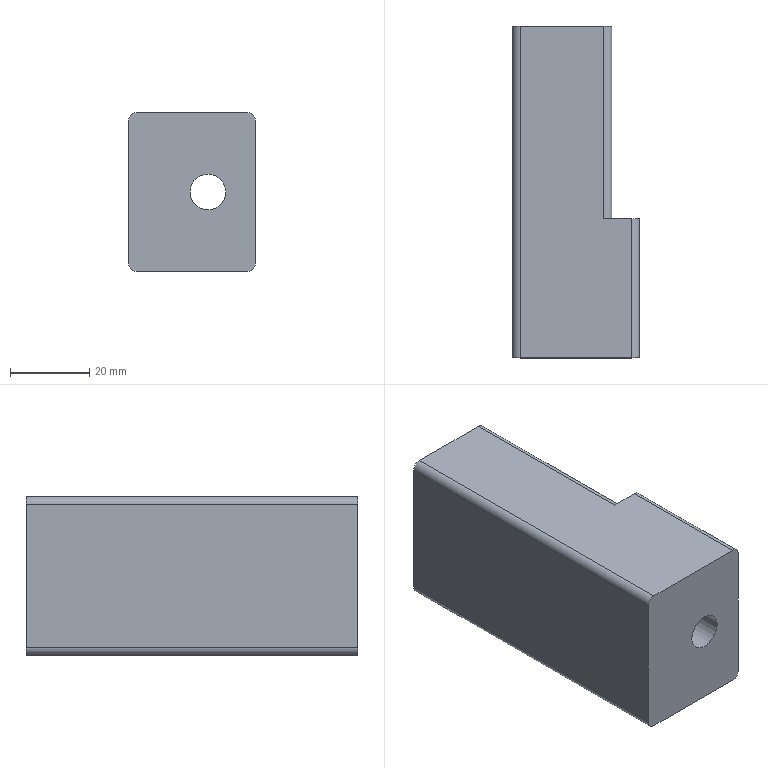NC program | Mastercam | posted with a generic post | part box 32 x 83.5 x 40 mm
Lines 1603 to 2565 of 4494:
(10 FEM |TOOL - 9|DIA. OFF. - 9|LEN. - 9|TOOL DIA. - 10.)
N3262 T9 M6
N3264 G0 G54 G90 X.244 Y-22.653 C0. B0. S7000 M3
N3266 G43 H9 Z50.
N3268 Z1.
N3270 G1 Z-.499 F600.
N3272 X4.744 Y-5.225 F3000.
N3274 G3 X4.9 Y-4. I-4.744 J1.225
N3276 X0. Y.9 I-4.9
N3278 X-4.9 Y-4. J-4.9
N3280 X-4.744 Y-5.225 I4.9
N3282 G1 X-.244 Y-22.653
N3284 Z-.998 F600.
N3286 X-4.744 Y-5.225 F3000.
N3288 G2 X-4.9 Y-4. I4.744 J1.225
N3290 X0. Y.9 I4.9
N3292 X4.9 Y-4. J-4.9
N3294 X4.744 Y-5.225 I-4.9
N3296 G1 X.244 Y-22.653
N3298 Z-1.497 F600.
N3300 X4.744 Y-5.225 F3000.
N3302 G3 X4.9 Y-4. I-4.744 J1.225
N3304 X0. Y.9 I-4.9
N3306 X-4.9 Y-4. J-4.9
N3308 X-4.744 Y-5.225 I4.9
N3310 G1 X-.244 Y-22.653
N3312 Z-1.996 F600.
N3314 X-4.744 Y-5.225 F3000.
N3316 G2 X-4.9 Y-4. I4.744 J1.225
N3318 X0. Y.9 I4.9
N3320 X4.9 Y-4. J-4.9
N3322 X4.744 Y-5.225 I-4.9
N3324 G1 X.244 Y-22.653
N3326 Z-2.495 F600.
N3328 X4.744 Y-5.225 F3000.
N3330 G3 X4.9 Y-4. I-4.744 J1.225
N3332 X0. Y.9 I-4.9
N3334 X-4.9 Y-4. J-4.9
N3336 X-4.744 Y-5.225 I4.9
N3338 G1 X-.244 Y-22.653
N3340 Z-2.994 F600.
N3342 X-4.744 Y-5.225 F3000.
N3344 G2 X-4.9 Y-4. I4.744 J1.225
N3346 X0. Y.9 I4.9
N3348 X4.9 Y-4. J-4.9
N3350 X4.744 Y-5.225 I-4.9
N3352 G1 X.244 Y-22.653
N3354 Z-3.493 F600.
N3356 X4.744 Y-5.225 F3000.
N3358 G3 X4.9 Y-4. I-4.744 J1.225
N3360 X0. Y.9 I-4.9
N3362 X-4.9 Y-4. J-4.9
N3364 X-4.744 Y-5.225 I4.9
N3366 G1 X-.244 Y-22.653
N3368 Z-3.992 F600.
N3370 X-4.744 Y-5.225 F3000.
N3372 G2 X-4.9 Y-4. I4.744 J1.225
N3374 X0. Y.9 I4.9
N3376 X4.9 Y-4. J-4.9
N3378 X4.744 Y-5.225 I-4.9
N3380 G1 X.244 Y-22.653
N3382 Z-4.491 F600.
N3384 X4.744 Y-5.225 F3000.
N3386 G3 X4.9 Y-4. I-4.744 J1.225
N3388 X0. Y.9 I-4.9
N3390 X-4.9 Y-4. J-4.9
N3392 X-4.744 Y-5.225 I4.9
N3394 G1 X-.244 Y-22.653
N3396 Z-4.99 F600.
N3398 X-4.744 Y-5.225 F3000.
N3400 G2 X-4.9 Y-4. I4.744 J1.225
N3402 X0. Y.9 I4.9
N3404 X4.9 Y-4. J-4.9
N3406 X4.744 Y-5.225 I-4.9
N3408 G1 X.244 Y-22.653
N3410 Z-5.489 F600.
N3412 X4.744 Y-5.225 F3000.
N3414 G3 X4.9 Y-4. I-4.744 J1.225
N3416 X0. Y.9 I-4.9
N3418 X-4.9 Y-4. J-4.9
N3420 X-4.744 Y-5.225 I4.9
N3422 G1 X-.244 Y-22.653
N3424 Z-5.988 F600.
N3426 X-4.744 Y-5.225 F3000.
N3428 G2 X-4.9 Y-4. I4.744 J1.225
N3430 X0. Y.9 I4.9
N3432 X4.9 Y-4. J-4.9
N3434 X4.744 Y-5.225 I-4.9
N3436 G1 X.244 Y-22.653
N3438 Z-6.487 F600.
N3440 X4.744 Y-5.225 F3000.
N3442 G3 X4.9 Y-4. I-4.744 J1.225
N3444 X0. Y.9 I-4.9
N3446 X-4.9 Y-4. J-4.9
N3448 X-4.744 Y-5.225 I4.9
N3450 G1 X-.244 Y-22.653
N3452 Z-6.986 F600.
N3454 X-4.744 Y-5.225 F3000.
N3456 G2 X-4.9 Y-4. I4.744 J1.225
N3458 X0. Y.9 I4.9
N3460 X4.9 Y-4. J-4.9
N3462 X4.744 Y-5.225 I-4.9
N3464 G1 X.244 Y-22.653
N3466 Z-7.485 F600.
N3468 X4.744 Y-5.225 F3000.
N3470 G3 X4.9 Y-4. I-4.744 J1.225
N3472 X0. Y.9 I-4.9
N3474 X-4.9 Y-4. J-4.9
N3476 X-4.744 Y-5.225 I4.9
N3478 G1 X-.244 Y-22.653
N3480 Z-7.984 F600.
N3482 X-4.744 Y-5.225 F3000.
N3484 G2 X-4.9 Y-4. I4.744 J1.225
N3486 X0. Y.9 I4.9
N3488 X4.9 Y-4. J-4.9
N3490 X4.744 Y-5.225 I-4.9
N3492 G1 X.244 Y-22.653
N3494 Z-8.482 F600.
N3496 X4.744 Y-5.225 F3000.
N3498 G3 X4.9 Y-4. I-4.744 J1.225
N3500 X0. Y.9 I-4.9
N3502 X-4.9 Y-4. J-4.9
N3504 X-4.744 Y-5.225 I4.9
N3506 G1 X-.244 Y-22.653
N3508 Z-8.981 F600.
N3510 X-4.744 Y-5.225 F3000.
N3512 G2 X-4.9 Y-4. I4.744 J1.225
N3514 X0. Y.9 I4.9
N3516 X4.9 Y-4. J-4.9
N3518 X4.744 Y-5.225 I-4.9
N3520 G1 X.244 Y-22.653
N3522 Z-9.48 F600.
N3524 X4.744 Y-5.225 F3000.
N3526 G3 X4.9 Y-4. I-4.744 J1.225
N3528 X0. Y.9 I-4.9
N3530 X-4.9 Y-4. J-4.9
N3532 X-4.744 Y-5.225 I4.9
N3534 G1 X-.244 Y-22.653
N3536 Z-9.979 F600.
N3538 X-4.744 Y-5.225 F3000.
N3540 G2 X-4.9 Y-4. I4.744 J1.225
N3542 X0. Y.9 I4.9
N3544 X4.9 Y-4. J-4.9
N3546 X4.744 Y-5.225 I-4.9
N3548 G1 X.244 Y-22.653
N3550 Z-10.478 F600.
N3552 X4.744 Y-5.225 F3000.
N3554 G3 X4.9 Y-4. I-4.744 J1.225
N3556 X0. Y.9 I-4.9
N3558 X-4.9 Y-4. J-4.9
N3560 X-4.744 Y-5.225 I4.9
N3562 G1 X-.244 Y-22.653
N3564 Z-10.977 F600.
N3566 X-4.744 Y-5.225 F3000.
N3568 G2 X-4.9 Y-4. I4.744 J1.225
N3570 X0. Y.9 I4.9
N3572 X4.9 Y-4. J-4.9
N3574 X4.744 Y-5.225 I-4.9
N3576 G1 X.244 Y-22.653
N3578 Z-11.476 F600.
N3580 X4.744 Y-5.225 F3000.
N3582 G3 X4.9 Y-4. I-4.744 J1.225
N3584 X0. Y.9 I-4.9
N3586 X-4.9 Y-4. J-4.9
N3588 X-4.744 Y-5.225 I4.9
N3590 G1 X-.244 Y-22.653
N3592 Z-11.975 F600.
N3594 X-4.744 Y-5.225 F3000.
N3596 G2 X-4.9 Y-4. I4.744 J1.225
N3598 X0. Y.9 I4.9
N3600 X4.9 Y-4. J-4.9
N3602 X4.744 Y-5.225 I-4.9
N3604 G1 X.244 Y-22.653
N3606 Z-12.474 F600.
N3608 X4.744 Y-5.225 F3000.
N3610 G3 X4.9 Y-4. I-4.744 J1.225
N3612 X0. Y.9 I-4.9
N3614 X-4.9 Y-4. J-4.9
N3616 X-4.744 Y-5.225 I4.9
N3618 G1 X-.244 Y-22.653
N3620 Z-12.973 F600.
N3622 X-4.744 Y-5.225 F3000.
N3624 G2 X-4.9 Y-4. I4.744 J1.225
N3626 X0. Y.9 I4.9
N3628 X4.9 Y-4. J-4.9
N3630 X4.744 Y-5.225 I-4.9
N3632 G1 X.244 Y-22.653
N3634 Z-13.472 F600.
N3636 X4.744 Y-5.225 F3000.
N3638 G3 X4.9 Y-4. I-4.744 J1.225
N3640 X0. Y.9 I-4.9
N3642 X-4.9 Y-4. J-4.9
N3644 X-4.744 Y-5.225 I4.9
N3646 G1 X-.244 Y-22.653
N3648 Z-13.971 F600.
N3650 X-4.744 Y-5.225 F3000.
N3652 G2 X-4.9 Y-4. I4.744 J1.225
N3654 X0. Y.9 I4.9
N3656 X4.9 Y-4. J-4.9
N3658 X4.744 Y-5.225 I-4.9
N3660 G1 X.244 Y-22.653
N3662 Z-14.47 F600.
N3664 X4.744 Y-5.225 F3000.
N3666 G3 X4.9 Y-4. I-4.744 J1.225
N3668 X0. Y.9 I-4.9
N3670 X-4.9 Y-4. J-4.9
N3672 X-4.744 Y-5.225 I4.9
N3674 G1 X-.244 Y-22.653
N3676 Z-14.969 F600.
N3678 X-4.744 Y-5.225 F3000.
N3680 G2 X-4.9 Y-4. I4.744 J1.225
N3682 X0. Y.9 I4.9
N3684 X4.9 Y-4. J-4.9
N3686 X4.744 Y-5.225 I-4.9
N3688 G1 X.244 Y-22.653
N3690 Z-15.468 F600.
N3692 X4.744 Y-5.225 F3000.
N3694 G3 X4.9 Y-4. I-4.744 J1.225
N3696 X0. Y.9 I-4.9
N3698 X-4.9 Y-4. J-4.9
N3700 X-4.744 Y-5.225 I4.9
N3702 G1 X-.244 Y-22.653
N3704 Z-15.967 F600.
N3706 X-4.744 Y-5.225 F3000.
N3708 G2 X-4.9 Y-4. I4.744 J1.225
N3710 X0. Y.9 I4.9
N3712 X4.9 Y-4. J-4.9
N3714 X4.744 Y-5.225 I-4.9
N3716 G1 X.244 Y-22.653
N3718 Z-16.466 F600.
N3720 X4.744 Y-5.225 F3000.
N3722 G3 X4.9 Y-4. I-4.744 J1.225
N3724 X0. Y.9 I-4.9
N3726 X-4.9 Y-4. J-4.9
N3728 X-4.744 Y-5.225 I4.9
N3730 G1 X-.244 Y-22.653
N3732 Z-16.965 F600.
N3734 X-4.744 Y-5.225 F3000.
N3736 G2 X-4.9 Y-4. I4.744 J1.225
N3738 X0. Y.9 I4.9
N3740 X4.9 Y-4. J-4.9
N3742 X4.744 Y-5.225 I-4.9
N3744 G1 X.244 Y-22.653
N3746 Z-17.464 F600.
N3748 X4.744 Y-5.225 F3000.
N3750 G3 X4.9 Y-4. I-4.744 J1.225
N3752 X0. Y.9 I-4.9
N3754 X-4.9 Y-4. J-4.9
N3756 X-4.744 Y-5.225 I4.9
N3758 G1 X-.244 Y-22.653
N3760 Z-17.963 F600.
N3762 X-4.744 Y-5.225 F3000.
N3764 G2 X-4.9 Y-4. I4.744 J1.225
N3766 X0. Y.9 I4.9
N3768 X4.9 Y-4. J-4.9
N3770 X4.744 Y-5.225 I-4.9
N3772 G1 X.244 Y-22.653
N3774 Z-18.462 F600.
N3776 X4.744 Y-5.225 F3000.
N3778 G3 X4.9 Y-4. I-4.744 J1.225
N3780 X0. Y.9 I-4.9
N3782 X-4.9 Y-4. J-4.9
N3784 X-4.744 Y-5.225 I4.9
N3786 G1 X-.244 Y-22.653
N3788 Z-18.961 F600.
N3790 X-4.744 Y-5.225 F3000.
N3792 G2 X-4.9 Y-4. I4.744 J1.225
N3794 X0. Y.9 I4.9
N3796 X4.9 Y-4. J-4.9
N3798 X4.744 Y-5.225 I-4.9
N3800 G1 X.244 Y-22.653
N3802 Z-19.46 F600.
N3804 X4.744 Y-5.225 F3000.
N3806 G3 X4.9 Y-4. I-4.744 J1.225
N3808 X0. Y.9 I-4.9
N3810 X-4.9 Y-4. J-4.9
N3812 X-4.744 Y-5.225 I4.9
N3814 G1 X-.244 Y-22.653
N3816 Z-19.959 F600.
N3818 X-4.744 Y-5.225 F3000.
N3820 G2 X-4.9 Y-4. I4.744 J1.225
N3822 X0. Y.9 I4.9
N3824 X4.9 Y-4. J-4.9
N3826 X4.744 Y-5.225 I-4.9
N3828 G1 X.244 Y-22.653
N3830 Z-20.458 F600.
N3832 X4.744 Y-5.225 F3000.
N3834 G3 X4.9 Y-4. I-4.744 J1.225
N3836 X0. Y.9 I-4.9
N3838 X-4.9 Y-4. J-4.9
N3840 X-4.744 Y-5.225 I4.9
N3842 G1 X-.244 Y-22.653
N3844 Z-20.957 F600.
N3846 X-4.744 Y-5.225 F3000.
N3848 G2 X-4.9 Y-4. I4.744 J1.225
N3850 X0. Y.9 I4.9
N3852 X4.9 Y-4. J-4.9
N3854 X4.744 Y-5.225 I-4.9
N3856 G1 X.244 Y-22.653
N3858 Z-21.456 F600.
N3860 X4.744 Y-5.225 F3000.
N3862 G3 X4.9 Y-4. I-4.744 J1.225
N3864 X0. Y.9 I-4.9
N3866 X-4.9 Y-4. J-4.9
N3868 X-4.744 Y-5.225 I4.9
N3870 G1 X-.244 Y-22.653
N3872 Z-21.955 F600.
N3874 X-4.744 Y-5.225 F3000.
N3876 G2 X-4.9 Y-4. I4.744 J1.225
N3878 X0. Y.9 I4.9
N3880 X4.9 Y-4. J-4.9
N3882 X4.744 Y-5.225 I-4.9
N3884 G1 X.244 Y-22.653
N3886 Z-22.454 F600.
N3888 X4.744 Y-5.225 F3000.
N3890 G3 X4.9 Y-4. I-4.744 J1.225
N3892 X0. Y.9 I-4.9
N3894 X-4.9 Y-4. J-4.9
N3896 X-4.744 Y-5.225 I4.9
N3898 G1 X-.244 Y-22.653
N3900 Z-22.953 F600.
N3902 X-4.744 Y-5.225 F3000.
N3904 G2 X-4.9 Y-4. I4.744 J1.225
N3906 X0. Y.9 I4.9
N3908 X4.9 Y-4. J-4.9
N3910 X4.744 Y-5.225 I-4.9
N3912 G1 X.244 Y-22.653
N3914 Z-23.452 F600.
N3916 X4.744 Y-5.225 F3000.
N3918 G3 X4.9 Y-4. I-4.744 J1.225
N3920 X0. Y.9 I-4.9
N3922 X-4.9 Y-4. J-4.9
N3924 X-4.744 Y-5.225 I4.9
N3926 G1 X-.244 Y-22.653
N3928 Z-23.951 F600.
N3930 X-4.744 Y-5.225 F3000.
N3932 G2 X-4.9 Y-4. I4.744 J1.225
N3934 X0. Y.9 I4.9
N3936 X4.9 Y-4. J-4.9
N3938 X4.744 Y-5.225 I-4.9
N3940 G1 X.244 Y-22.653
N3942 Z-24.449 F600.
N3944 X4.744 Y-5.225 F3000.
N3946 G3 X4.9 Y-4. I-4.744 J1.225
N3948 X0. Y.9 I-4.9
N3950 X-4.9 Y-4. J-4.9
N3952 X-4.744 Y-5.225 I4.9
N3954 G1 X-.244 Y-22.653
N3956 Z-24.948 F600.
N3958 X-4.744 Y-5.225 F3000.
N3960 G2 X-4.9 Y-4. I4.744 J1.225
N3962 X0. Y.9 I4.9
N3964 X4.9 Y-4. J-4.9
N3966 X4.744 Y-5.225 I-4.9
N3968 G1 X.244 Y-22.653
N3970 Z-25.447 F600.
N3972 X4.744 Y-5.225 F3000.
N3974 G3 X4.9 Y-4. I-4.744 J1.225
N3976 X0. Y.9 I-4.9
N3978 X-4.9 Y-4. J-4.9
N3980 X-4.744 Y-5.225 I4.9
N3982 G1 X-.244 Y-22.653
N3984 Z-25.946 F600.
N3986 X-4.744 Y-5.225 F3000.
N3988 G2 X-4.9 Y-4. I4.744 J1.225
N3990 X0. Y.9 I4.9
N3992 X4.9 Y-4. J-4.9
N3994 X4.744 Y-5.225 I-4.9
N3996 G1 X.244 Y-22.653
N3998 Z-26.445 F600.
N4000 X4.744 Y-5.225 F3000.
N4002 G3 X4.9 Y-4. I-4.744 J1.225
N4004 X0. Y.9 I-4.9
N4006 X-4.9 Y-4. J-4.9
N4008 X-4.744 Y-5.225 I4.9
N4010 G1 X-.244 Y-22.653
N4012 Z-26.944 F600.
N4014 X-4.744 Y-5.225 F3000.
N4016 G2 X-4.9 Y-4. I4.744 J1.225
N4018 X0. Y.9 I4.9
N4020 X4.9 Y-4. J-4.9
N4022 X4.744 Y-5.225 I-4.9
N4024 G1 X.244 Y-22.653
N4026 Z-27.443 F600.
N4028 X4.744 Y-5.225 F3000.
N4030 G3 X4.9 Y-4. I-4.744 J1.225
N4032 X0. Y.9 I-4.9
N4034 X-4.9 Y-4. J-4.9
N4036 X-4.744 Y-5.225 I4.9
N4038 G1 X-.244 Y-22.653
N4040 Z-27.942 F600.
N4042 X-4.744 Y-5.225 F3000.
N4044 G2 X-4.9 Y-4. I4.744 J1.225
N4046 X0. Y.9 I4.9
N4048 X4.9 Y-4. J-4.9
N4050 X4.744 Y-5.225 I-4.9
N4052 G1 X.244 Y-22.653
N4054 Z-28.441 F600.
N4056 X4.744 Y-5.225 F3000.
N4058 G3 X4.9 Y-4. I-4.744 J1.225
N4060 X0. Y.9 I-4.9
N4062 X-4.9 Y-4. J-4.9
N4064 X-4.744 Y-5.225 I4.9
N4066 G1 X-.244 Y-22.653
N4068 Z-28.94 F600.
N4070 X-4.744 Y-5.225 F3000.
N4072 G2 X-4.9 Y-4. I4.744 J1.225
N4074 X0. Y.9 I4.9
N4076 X4.9 Y-4. J-4.9
N4078 X4.744 Y-5.225 I-4.9
N4080 G1 X.244 Y-22.653
N4082 Z-29.439 F600.
N4084 X4.744 Y-5.225 F3000.
N4086 G3 X4.9 Y-4. I-4.744 J1.225
N4088 X0. Y.9 I-4.9
N4090 X-4.9 Y-4. J-4.9
N4092 X-4.744 Y-5.225 I4.9
N4094 G1 X-.244 Y-22.653
N4096 Z-29.938 F600.
N4098 X-4.744 Y-5.225 F3000.
N4100 G2 X-4.9 Y-4. I4.744 J1.225
N4102 X0. Y.9 I4.9
N4104 X4.9 Y-4. J-4.9
N4106 X4.744 Y-5.225 I-4.9
N4108 G1 X.244 Y-22.653
N4110 Z-30.437 F600.
N4112 X4.744 Y-5.225 F3000.
N4114 G3 X4.9 Y-4. I-4.744 J1.225
N4116 X0. Y.9 I-4.9
N4118 X-4.9 Y-4. J-4.9
N4120 X-4.744 Y-5.225 I4.9
N4122 G1 X-.244 Y-22.653
N4124 Z-30.936 F600.
N4126 X-4.744 Y-5.225 F3000.
N4128 G2 X-4.9 Y-4. I4.744 J1.225
N4130 X0. Y.9 I4.9
N4132 X4.9 Y-4. J-4.9
N4134 X4.744 Y-5.225 I-4.9
N4136 G1 X.244 Y-22.653
N4138 Z-31.435 F600.
N4140 X4.744 Y-5.225 F3000.
N4142 G3 X4.9 Y-4. I-4.744 J1.225
N4144 X0. Y.9 I-4.9
N4146 X-4.9 Y-4. J-4.9
N4148 X-4.744 Y-5.225 I4.9
N4150 G1 X-.244 Y-22.653
N4152 Z-31.934 F600.
N4154 X-4.744 Y-5.225 F3000.
N4156 G2 X-4.9 Y-4. I4.744 J1.225
N4158 X0. Y.9 I4.9
N4160 X4.9 Y-4. J-4.9
N4162 X4.744 Y-5.225 I-4.9
N4164 G1 X.244 Y-22.653
N4166 Z-32.433 F600.
N4168 X4.744 Y-5.225 F3000.
N4170 G3 X4.9 Y-4. I-4.744 J1.225
N4172 X0. Y.9 I-4.9
N4174 X-4.9 Y-4. J-4.9
N4176 X-4.744 Y-5.225 I4.9
N4178 G1 X-.244 Y-22.653
N4180 Z-32.932 F600.
N4182 X-4.744 Y-5.225 F3000.
N4184 G2 X-4.9 Y-4. I4.744 J1.225
N4186 X0. Y.9 I4.9
N4188 X4.9 Y-4. J-4.9
N4190 X4.744 Y-5.225 I-4.9
N4192 G1 X.244 Y-22.653
N4194 Z-33.431 F600.
N4196 X4.744 Y-5.225 F3000.
N4198 G3 X4.9 Y-4. I-4.744 J1.225
N4200 X0. Y.9 I-4.9
N4202 X-4.9 Y-4. J-4.9
N4204 X-4.744 Y-5.225 I4.9
N4206 G1 X-.244 Y-22.653
N4208 Z-33.93 F600.
N4210 X-4.744 Y-5.225 F3000.
N4212 G2 X-4.9 Y-4. I4.744 J1.225
N4214 X0. Y.9 I4.9
N4216 X4.9 Y-4. J-4.9
N4218 X4.744 Y-5.225 I-4.9
N4220 G1 X.244 Y-22.653
N4222 Z-34.429 F600.
N4224 X4.744 Y-5.225 F3000.
N4226 G3 X4.9 Y-4. I-4.744 J1.225
N4228 X0. Y.9 I-4.9
N4230 X-4.9 Y-4. J-4.9
N4232 X-4.744 Y-5.225 I4.9
N4234 G1 X-.244 Y-22.653
N4236 Z-34.928 F600.
N4238 X-4.744 Y-5.225 F3000.
N4240 G2 X-4.9 Y-4. I4.744 J1.225
N4242 X0. Y.9 I4.9
N4244 X4.9 Y-4. J-4.9
N4246 X4.744 Y-5.225 I-4.9
N4248 G1 X.244 Y-22.653
N4250 Z-35.427 F600.
N4252 X4.744 Y-5.225 F3000.
N4254 G3 X4.9 Y-4. I-4.744 J1.225
N4256 X0. Y.9 I-4.9
N4258 X-4.9 Y-4. J-4.9
N4260 X-4.744 Y-5.225 I4.9
N4262 G1 X-.244 Y-22.653
N4264 Z-35.926 F600.
N4266 X-4.744 Y-5.225 F3000.
N4268 G2 X-4.9 Y-4. I4.744 J1.225
N4270 X0. Y.9 I4.9
N4272 X4.9 Y-4. J-4.9
N4274 X4.744 Y-5.225 I-4.9
N4276 G1 X.244 Y-22.653
N4278 Z-36.425 F600.
N4280 X4.744 Y-5.225 F3000.
N4282 G3 X4.9 Y-4. I-4.744 J1.225
N4284 X0. Y.9 I-4.9
N4286 X-4.9 Y-4. J-4.9
N4288 X-4.744 Y-5.225 I4.9
N4290 G1 X-.244 Y-22.653
N4292 Z-36.924 F600.
N4294 X-4.744 Y-5.225 F3000.
N4296 G2 X-4.9 Y-4. I4.744 J1.225
N4298 X0. Y.9 I4.9
N4300 X4.9 Y-4. J-4.9
N4302 X4.744 Y-5.225 I-4.9
N4304 G1 X.244 Y-22.653
N4306 Z-37.423 F600.
N4308 X4.744 Y-5.225 F3000.
N4310 G3 X4.9 Y-4. I-4.744 J1.225
N4312 X0. Y.9 I-4.9
N4314 X-4.9 Y-4. J-4.9
N4316 X-4.744 Y-5.225 I4.9
N4318 G1 X-.244 Y-22.653
N4320 Z-37.922 F600.
N4322 X-4.744 Y-5.225 F3000.
N4324 G2 X-4.9 Y-4. I4.744 J1.225
N4326 X0. Y.9 I4.9
N4328 X4.9 Y-4. J-4.9
N4330 X4.744 Y-5.225 I-4.9
N4332 G1 X.244 Y-22.653
N4334 Z-38.421 F600.
N4336 X4.744 Y-5.225 F3000.
N4338 G3 X4.9 Y-4. I-4.744 J1.225
N4340 X0. Y.9 I-4.9
N4342 X-4.9 Y-4. J-4.9
N4344 X-4.744 Y-5.225 I4.9
N4346 G1 X-.244 Y-22.653
N4348 Z-38.92 F600.
N4350 X-4.744 Y-5.225 F3000.
N4352 G2 X-4.9 Y-4. I4.744 J1.225
N4354 X0. Y.9 I4.9
N4356 X4.9 Y-4. J-4.9
N4358 X4.744 Y-5.225 I-4.9
N4360 G1 X.244 Y-22.653
N4362 Z-39.419 F600.
N4364 X4.744 Y-5.225 F3000.
N4366 G3 X4.9 Y-4. I-4.744 J1.225
N4368 X0. Y.9 I-4.9
N4370 X-4.9 Y-4. J-4.9
N4372 X-4.744 Y-5.225 I4.9
N4374 G1 X-.244 Y-22.653
N4376 Z-39.918 F600.
N4378 X-4.744 Y-5.225 F3000.
N4380 G2 X-4.9 Y-4. I4.744 J1.225
N4382 X0. Y.9 I4.9
N4384 X4.9 Y-4. J-4.9
N4386 X4.744 Y-5.225 I-4.9
N4388 G1 X.244 Y-22.653
N4390 Z-40.416 F600.
N4392 X4.744 Y-5.225 F3000.
N4394 G3 X4.9 Y-4. I-4.744 J1.225
N4396 X0. Y.9 I-4.9
N4398 X-4.9 Y-4. J-4.9
N4400 X-4.744 Y-5.225 I4.9
N4402 G1 X-.244 Y-22.653
N4404 Z-40.915 F600.
N4406 X-4.744 Y-5.225 F3000.
N4408 G2 X-4.9 Y-4. I4.744 J1.225
N4410 X0. Y.9 I4.9
N4412 X4.9 Y-4. J-4.9
N4414 X4.744 Y-5.225 I-4.9
N4416 G1 X.244 Y-22.653
N4418 Z-41.414 F600.
N4420 X4.744 Y-5.225 F3000.
N4422 G3 X4.9 Y-4. I-4.744 J1.225
N4424 X0. Y.9 I-4.9
N4426 X-4.9 Y-4. J-4.9
N4428 X-4.744 Y-5.225 I4.9
N4430 G1 X-.244 Y-22.653
N4432 Z-41.913 F600.
N4434 X-4.744 Y-5.225 F3000.
N4436 G2 X-4.9 Y-4. I4.744 J1.225
N4438 X0. Y.9 I4.9
N4440 X4.9 Y-4. J-4.9
N4442 X4.744 Y-5.225 I-4.9
N4444 G1 X.244 Y-22.653
N4446 Z-42.412 F600.
N4448 X4.744 Y-5.225 F3000.
N4450 G3 X4.9 Y-4. I-4.744 J1.225
N4452 X0. Y.9 I-4.9
N4454 X-4.9 Y-4. J-4.9
N4456 X-4.744 Y-5.225 I4.9
N4458 G1 X-.244 Y-22.653
N4460 Z-42.911 F600.
N4462 X-4.744 Y-5.225 F3000.
N4464 G2 X-4.9 Y-4. I4.744 J1.225
N4466 X0. Y.9 I4.9
N4468 X4.9 Y-4. J-4.9
N4470 X4.744 Y-5.225 I-4.9
N4472 G1 X.244 Y-22.653
N4474 Z-43.41 F600.
N4476 X4.744 Y-5.225 F3000.
N4478 G3 X4.9 Y-4. I-4.744 J1.225
N4480 X0. Y.9 I-4.9
N4482 X-4.9 Y-4. J-4.9
N4484 X-4.744 Y-5.225 I4.9
N4486 G1 X-.244 Y-22.653
N4488 Z-43.909 F600.
N4490 X-4.744 Y-5.225 F3000.
N4492 G2 X-4.9 Y-4. I4.744 J1.225
N4494 X0. Y.9 I4.9
N4496 X4.9 Y-4. J-4.9
N4498 X4.744 Y-5.225 I-4.9
N4500 G1 X.244 Y-22.653
N4502 Z-44.408 F600.
N4504 X4.744 Y-5.225 F3000.
N4506 G3 X4.9 Y-4. I-4.744 J1.225
N4508 X0. Y.9 I-4.9
N4510 X-4.9 Y-4. J-4.9
N4512 X-4.744 Y-5.225 I4.9
N4514 G1 X-.244 Y-22.653
N4516 Z-44.907 F600.
N4518 X-4.744 Y-5.225 F3000.
N4520 G2 X-4.9 Y-4. I4.744 J1.225
N4522 X0. Y.9 I4.9
N4524 X4.9 Y-4. J-4.9
N4526 X4.744 Y-5.225 I-4.9
N4528 G1 X.244 Y-22.653
N4530 Z-45.406 F600.
N4532 X4.744 Y-5.225 F3000.
N4534 G3 X4.9 Y-4. I-4.744 J1.225
N4536 X0. Y.9 I-4.9
N4538 X-4.9 Y-4. J-4.9
N4540 X-4.744 Y-5.225 I4.9
N4542 G1 X-.244 Y-22.653
N4544 Z-45.905 F600.
N4546 X-4.744 Y-5.225 F3000.
N4548 G2 X-4.9 Y-4. I4.744 J1.225
N4550 X0. Y.9 I4.9
N4552 X4.9 Y-4. J-4.9
N4554 X4.744 Y-5.225 I-4.9
N4556 G1 X.244 Y-22.653
N4558 Z-46.404 F600.
N4560 X4.744 Y-5.225 F3000.
N4562 G3 X4.9 Y-4. I-4.744 J1.225
N4564 X0. Y.9 I-4.9
N4566 X-4.9 Y-4. J-4.9
N4568 X-4.744 Y-5.225 I4.9
N4570 G1 X-.244 Y-22.653
N4572 Z-46.903 F600.
N4574 X-4.744 Y-5.225 F3000.
N4576 G2 X-4.9 Y-4. I4.744 J1.225
N4578 X0. Y.9 I4.9
N4580 X4.9 Y-4. J-4.9
N4582 X4.744 Y-5.225 I-4.9
N4584 G1 X.244 Y-22.653
N4586 Z-47.402 F600.
N4588 X4.744 Y-5.225 F3000.
N4590 G3 X4.9 Y-4. I-4.744 J1.225
N4592 X0. Y.9 I-4.9
N4594 X-4.9 Y-4. J-4.9
N4596 X-4.744 Y-5.225 I4.9
N4598 G1 X-.244 Y-22.653
N4600 Z-47.901 F600.
N4602 X-4.744 Y-5.225 F3000.
N4604 G2 X-4.9 Y-4. I4.744 J1.225
N4606 X0. Y.9 I4.9
N4608 X4.9 Y-4. J-4.9
N4610 X4.744 Y-5.225 I-4.9
N4612 G1 X.244 Y-22.653
N4614 Z-48.4 F600.
N4616 X4.744 Y-5.225 F3000.
N4618 G3 X4.9 Y-4. I-4.744 J1.225
N4620 X0. Y.9 I-4.9
N4622 X-4.9 Y-4. J-4.9
N4624 X-4.744 Y-5.225 I4.9
N4626 G1 X-.244 Y-22.653
N4628 G0 Z50.
N4630 X27.1 Y-6.
N4632 Z1.
N4634 G1 Z-.499 F600.
N4636 X26.1 F3000.
N4638 G3 X25.1 Y-7. J-1.
N4640 G2 X18. Y-14.1 I-7.1
N4642 G1 X11.619
N4644 G2 X4.519 Y-7. J7.1
N4646 X4.744 Y-5.225 I7.1
N4648 G3 X4.9 Y-4. I-4.744 J1.225
N4650 X0. Y.9 I-4.9
N4652 X-4.9 Y-4. J-4.9
N4654 X-4.744 Y-5.225 I4.9
N4656 G2 X-4.519 Y-7. I-6.875 J-1.775
N4658 X-11.619 Y-14.1 I-7.1
N4660 G1 X-18.
N4662 G2 X-25.1 Y-7. J7.1
N4664 G3 X-26.1 Y-6. I-1.
N4666 G1 X-27.1
N4668 Z-.998 F600.
N4670 X-26.1 F3000.
N4672 G2 X-25.1 Y-7. J-1.
N4674 G3 X-18. Y-14.1 I7.1
N4676 G1 X-11.619
N4678 G3 X-4.519 Y-7. J7.1
N4680 X-4.744 Y-5.225 I-7.1
N4682 G2 X-4.9 Y-4. I4.744 J1.225
N4684 X0. Y.9 I4.9
N4686 X4.9 Y-4. J-4.9
N4688 X4.744 Y-5.225 I-4.9
N4690 G3 X4.519 Y-7. I6.875 J-1.775
N4692 X11.619 Y-14.1 I7.1
N4694 G1 X18.
N4696 G3 X25.1 Y-7. J7.1
N4698 G2 X26.1 Y-6. I1.
N4700 G1 X27.1
N4702 Z-1.497 F600.
N4704 X26.1 F3000.
N4706 G3 X25.1 Y-7. J-1.
N4708 G2 X18. Y-14.1 I-7.1
N4710 G1 X11.619
N4712 G2 X4.519 Y-7. J7.1
N4714 X4.744 Y-5.225 I7.1
N4716 G3 X4.9 Y-4. I-4.744 J1.225
N4718 X0. Y.9 I-4.9
N4720 X-4.9 Y-4. J-4.9
N4722 X-4.744 Y-5.225 I4.9
N4724 G2 X-4.519 Y-7. I-6.875 J-1.775
N4726 X-11.619 Y-14.1 I-7.1
N4728 G1 X-18.
N4730 G2 X-25.1 Y-7. J7.1
N4732 G3 X-26.1 Y-6. I-1.
N4734 G1 X-27.1
N4736 Z-1.996 F600.
N4738 X-26.1 F3000.
N4740 G2 X-25.1 Y-7. J-1.
N4742 G3 X-18. Y-14.1 I7.1
N4744 G1 X-11.619
N4746 G3 X-4.519 Y-7. J7.1
N4748 X-4.744 Y-5.225 I-7.1
N4750 G2 X-4.9 Y-4. I4.744 J1.225
N4752 X0. Y.9 I4.9
N4754 X4.9 Y-4. J-4.9
N4756 X4.744 Y-5.225 I-4.9
N4758 G3 X4.519 Y-7. I6.875 J-1.775
N4760 X11.619 Y-14.1 I7.1
N4762 G1 X18.
N4764 G3 X25.1 Y-7. J7.1
N4766 G2 X26.1 Y-6. I1.
N4768 G1 X27.1
N4770 Z-2.495 F600.
N4772 X26.1 F3000.
N4774 G3 X25.1 Y-7. J-1.
N4776 G2 X18. Y-14.1 I-7.1
N4778 G1 X11.619
N4780 G2 X4.519 Y-7. J7.1
N4782 X4.744 Y-5.225 I7.1
N4784 G3 X4.9 Y-4. I-4.744 J1.225
N4786 X0. Y.9 I-4.9
N4788 X-4.9 Y-4. J-4.9
N4790 X-4.744 Y-5.225 I4.9
N4792 G2 X-4.519 Y-7. I-6.875 J-1.775
N4794 X-11.619 Y-14.1 I-7.1
N4796 G1 X-18.
N4798 G2 X-25.1 Y-7. J7.1
N4800 G3 X-26.1 Y-6. I-1.
N4802 G1 X-27.1
N4804 Z-2.994 F600.
N4806 X-26.1 F3000.
N4808 G2 X-25.1 Y-7. J-1.
N4810 G3 X-18. Y-14.1 I7.1
N4812 G1 X-11.619
N4814 G3 X-4.519 Y-7. J7.1
N4816 X-4.744 Y-5.225 I-7.1
N4818 G2 X-4.9 Y-4. I4.744 J1.225
N4820 X0. Y.9 I4.9
N4822 X4.9 Y-4. J-4.9
N4824 X4.744 Y-5.225 I-4.9
N4826 G3 X4.519 Y-7. I6.875 J-1.775
N4828 X11.619 Y-14.1 I7.1
N4830 G1 X18.
N4832 G3 X25.1 Y-7. J7.1
N4834 G2 X26.1 Y-6. I1.
N4836 G1 X27.1
N4838 Z-3.493 F600.
N4840 X26.1 F3000.
N4842 G3 X25.1 Y-7. J-1.
N4844 G2 X18. Y-14.1 I-7.1
N4846 G1 X11.619
N4848 G2 X4.519 Y-7. J7.1
N4850 X4.744 Y-5.225 I7.1
N4852 G3 X4.9 Y-4. I-4.744 J1.225
N4854 X0. Y.9 I-4.9
N4856 X-4.9 Y-4. J-4.9
N4858 X-4.744 Y-5.225 I4.9
N4860 G2 X-4.519 Y-7. I-6.875 J-1.775
N4862 X-11.619 Y-14.1 I-7.1
N4864 G1 X-18.
N4866 G2 X-25.1 Y-7. J7.1
N4868 G3 X-26.1 Y-6. I-1.
N4870 G1 X-27.1
N4872 Z-3.992 F600.
N4874 X-26.1 F3000.
N4876 G2 X-25.1 Y-7. J-1.
N4878 G3 X-18. Y-14.1 I7.1
N4880 G1 X-11.619
N4882 G3 X-4.519 Y-7. J7.1
N4884 X-4.744 Y-5.225 I-7.1
N4886 G2 X-4.9 Y-4. I4.744 J1.225
N4888 X0. Y.9 I4.9
N4890 X4.9 Y-4. J-4.9
N4892 X4.744 Y-5.225 I-4.9
N4894 G3 X4.519 Y-7. I6.875 J-1.775
N4896 X11.619 Y-14.1 I7.1
N4898 G1 X18.
N4900 G3 X25.1 Y-7. J7.1
N4902 G2 X26.1 Y-6. I1.
N4904 G1 X27.1
N4906 Z-4.491 F600.
N4908 X26.1 F3000.
N4910 G3 X25.1 Y-7. J-1.
N4912 G2 X18. Y-14.1 I-7.1
N4914 G1 X11.619
N4916 G2 X4.519 Y-7. J7.1
N4918 X4.744 Y-5.225 I7.1
N4920 G3 X4.9 Y-4. I-4.744 J1.225
N4922 X0. Y.9 I-4.9
N4924 X-4.9 Y-4. J-4.9
N4926 X-4.744 Y-5.225 I4.9
N4928 G2 X-4.519 Y-7. I-6.875 J-1.775
N4930 X-11.619 Y-14.1 I-7.1
N4932 G1 X-18.
N4934 G2 X-25.1 Y-7. J7.1
N4936 G3 X-26.1 Y-6. I-1.
N4938 G1 X-27.1
N4940 Z-4.99 F600.
N4942 X-26.1 F3000.
N4944 G2 X-25.1 Y-7. J-1.
N4946 G3 X-18. Y-14.1 I7.1
N4948 G1 X-11.619
N4950 G3 X-4.519 Y-7. J7.1
N4952 X-4.744 Y-5.225 I-7.1
N4954 G2 X-4.9 Y-4. I4.744 J1.225
N4956 X0. Y.9 I4.9
N4958 X4.9 Y-4. J-4.9
N4960 X4.744 Y-5.225 I-4.9
N4962 G3 X4.519 Y-7. I6.875 J-1.775
N4964 X11.619 Y-14.1 I7.1
N4966 G1 X18.
N4968 G3 X25.1 Y-7. J7.1
N4970 G2 X26.1 Y-6. I1.
N4972 G1 X27.1
N4974 Z-5.489 F600.
N4976 X26.1 F3000.
N4978 G3 X25.1 Y-7. J-1.
N4980 G2 X18. Y-14.1 I-7.1
N4982 G1 X11.619
N4984 G2 X4.519 Y-7. J7.1
N4986 X4.744 Y-5.225 I7.1
N4988 G3 X4.9 Y-4. I-4.744 J1.225
N4990 X0. Y.9 I-4.9
N4992 X-4.9 Y-4. J-4.9
N4994 X-4.744 Y-5.225 I4.9
N4996 G2 X-4.519 Y-7. I-6.875 J-1.775
N4998 X-11.619 Y-14.1 I-7.1
N5000 G1 X-18.
N5002 G2 X-25.1 Y-7. J7.1
N5004 G3 X-26.1 Y-6. I-1.
N5006 G1 X-27.1
N5008 Z-5.988 F600.
N5010 X-26.1 F3000.
N5012 G2 X-25.1 Y-7. J-1.
N5014 G3 X-18. Y-14.1 I7.1
N5016 G1 X-11.619
N5018 G3 X-4.519 Y-7. J7.1
N5020 X-4.744 Y-5.225 I-7.1
N5022 G2 X-4.9 Y-4. I4.744 J1.225
N5024 X0. Y.9 I4.9
N5026 X4.9 Y-4. J-4.9
N5028 X4.744 Y-5.225 I-4.9
N5030 G3 X4.519 Y-7. I6.875 J-1.775
N5032 X11.619 Y-14.1 I7.1
N5034 G1 X18.
N5036 G3 X25.1 Y-7. J7.1
N5038 G2 X26.1 Y-6. I1.
N5040 G1 X27.1
N5042 Z-6.487 F600.
N5044 X26.1 F3000.
N5046 G3 X25.1 Y-7. J-1.
N5048 G2 X18. Y-14.1 I-7.1
N5050 G1 X11.619
N5052 G2 X4.519 Y-7. J7.1
N5054 X4.744 Y-5.225 I7.1
N5056 G3 X4.9 Y-4. I-4.744 J1.225
N5058 X0. Y.9 I-4.9
N5060 X-4.9 Y-4. J-4.9
N5062 X-4.744 Y-5.225 I4.9
N5064 G2 X-4.519 Y-7. I-6.875 J-1.775
N5066 X-11.619 Y-14.1 I-7.1
N5068 G1 X-18.
N5070 G2 X-25.1 Y-7. J7.1
N5072 G3 X-26.1 Y-6. I-1.
N5074 G1 X-27.1
N5076 Z-6.986 F600.
N5078 X-26.1 F3000.
N5080 G2 X-25.1 Y-7. J-1.
N5082 G3 X-18. Y-14.1 I7.1
N5084 G1 X-11.619
N5086 G3 X-4.519 Y-7. J7.1
N5088 X-4.744 Y-5.225 I-7.1
N5090 G2 X-4.9 Y-4. I4.744 J1.225
N5092 X0. Y.9 I4.9
N5094 X4.9 Y-4. J-4.9
N5096 X4.744 Y-5.225 I-4.9
N5098 G3 X4.519 Y-7. I6.875 J-1.775
N5100 X11.619 Y-14.1 I7.1
N5102 G1 X18.
N5104 G3 X25.1 Y-7. J7.1
N5106 G2 X26.1 Y-6. I1.
N5108 G1 X27.1
N5110 Z-7.485 F600.
N5112 X26.1 F3000.
N5114 G3 X25.1 Y-7. J-1.
N5116 G2 X18. Y-14.1 I-7.1
N5118 G1 X11.619
N5120 G2 X4.519 Y-7. J7.1
N5122 X4.744 Y-5.225 I7.1
N5124 G3 X4.9 Y-4. I-4.744 J1.225
N5126 X0. Y.9 I-4.9
N5128 X-4.9 Y-4. J-4.9
N5130 X-4.744 Y-5.225 I4.9
N5132 G2 X-4.519 Y-7. I-6.875 J-1.775
N5134 X-11.619 Y-14.1 I-7.1
N5136 G1 X-18.
N5138 G2 X-25.1 Y-7. J7.1
N5140 G3 X-26.1 Y-6. I-1.
N5142 G1 X-27.1
N5144 Z-7.984 F600.
N5146 X-26.1 F3000.
N5148 G2 X-25.1 Y-7. J-1.
N5150 G3 X-18. Y-14.1 I7.1
N5152 G1 X-11.619
N5154 G3 X-4.519 Y-7. J7.1
N5156 X-4.744 Y-5.225 I-7.1
N5158 G2 X-4.9 Y-4. I4.744 J1.225
N5160 X0. Y.9 I4.9
N5162 X4.9 Y-4. J-4.9
N5164 X4.744 Y-5.225 I-4.9
N5166 G3 X4.519 Y-7. I6.875 J-1.775
N5168 X11.619 Y-14.1 I7.1
N5170 G1 X18.
N5172 G3 X25.1 Y-7. J7.1
N5174 G2 X26.1 Y-6. I1.
N5176 G1 X27.1
N5178 Z-8.482 F600.
N5180 X26.1 F3000.
N5182 G3 X25.1 Y-7. J-1.
N5184 G2 X18. Y-14.1 I-7.1